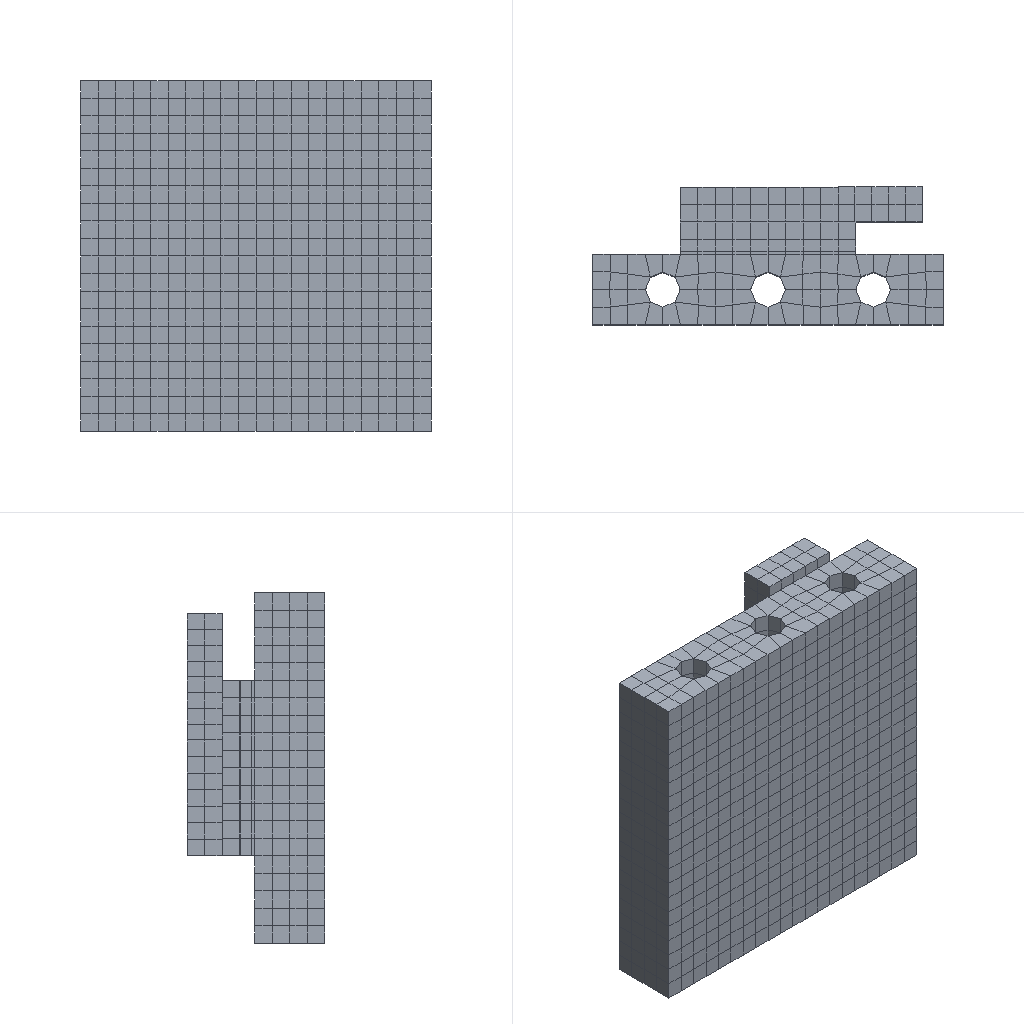Simulation study | ansys workbench
Set-up summary:
category,name,step,type,value,unit,region
solver,ansys_workbench
units,SI m-kg-s (Pa),,stated,"/units,MKS"
analysis,LS1,,steady-state thermal
load_step,LS1,LS1,steady-state thermal,nsubst=1; time=1
mesh,nodes,,,12761
mesh,elements,,,5722
element_type,SOLID279,,,2036
element_type,SURF152,,,1276
element_type,TARGE170,,,1205
element_type,CONTA174,,,1205
material,Cu,,E,1.15e+11,Pa
material,Cu,,nu,0.34
material,Cu,,density,8960,kg m^-3
material,Cu,,conductivity,397,W m^-1 C^-1
material,Cu,,specific_heat,385,J kg^-1 C^-1
material,Cu,,cte,1.75e-05,C^-1
material,?,,E,3.25e+11,Pa
material,?,,nu,0.29
material,?,,density,10220,kg m^-3
material,?,,conductivity,138,W m^-1 C^-1
material,?,,specific_heat,251,J kg^-1 C^-1
material,?,,cte,5.1e-06,C^-1
material,Ag,,E,8.3e+10,Pa
material,Ag,,nu,0.37
material,Ag,,density,10490,kg m^-3
material,Ag,,conductivity,429,W m^-1 C^-1
material,Ag,,specific_heat,237,J kg^-1 C^-1
material,Ag,,cte,1.89e-05,C^-1
material,SiC,,E,4.1e+11,Pa
material,SiC,,nu,0.25
material,SiC,,density,3200,kg m^-3
material,SiC,,conductivity,490,W m^-1 C^-1
material,SiC,,specific_heat,840,J kg^-1 C^-1
material,SiC,,cte,4.5e-06,C^-1
load,Define Uniform Initial temperature,model,body load temp,22,,all
load,"Create ""?""",LS1,heat flux,400000,,SURF152 #19
load,"Create ""______""",LS1,convection,15,,SURF152 #20
load,"Create ""______ 2""",LS1,convection,1000,,SURF152 #21
contact,Contact Region,,bonded (always),element=CONTA174
contact,Contact Region 2,,bonded (always),element=CONTA174
contact,Contact Region 3,,bonded (always),element=CONTA174
contact,Contact Region 4,,bonded (always),element=CONTA174
contact,Contact Region 5,,bonded (always),element=CONTA174
contact,Contact Region 6,,bonded (always),element=CONTA174
Ansys APDL input file, long lists of numbers shortened:
/batch
/config,noeldb,1     ! force off writing results to database
*get,_wallstrt,active,,time,wall
! ANSYS input file written by Workbench version 2021 R1
! File used for geometry attach:
/title,wbnew--___ (B5)
! ****** Begin Custom Load Command Snippet ******
/COM, ACT Extensions:
/COM,     LSDYNA, 2021.1
/COM,
! ****** End   Custom Load Command Snippet ******
*DIM,_wb_ProjectScratch_dir,string,248
_wb_ProjectScratch_dir(1) = ''
*DIM,_wb_SolverFiles_dir,string,248
_wb_SolverFiles_dir(1) = ''
*DIM,_wb_userfiles_dir,string,248
_wb_userfiles_dir(1) = ''
/com,--- Data in consistent MKS units. See Solving Units in the help system for more information.
/units,MKS
/nopr
/wb,file,start              !  signify a WB generated input file
/prep7
! Turn off shape checking because checks already performed inside WB mesher.
! See help system for more information.
SHPP,OFF,,NOWARN
/nolist
etcon,set             ! allow ANSYS to choose best KEYOP's for 180x elements, resets any applicable keyopt to MAPDL defaults
/com,*********** Nodes for the whole assembly ***********
nblock,3,,14037
(1i9,3e20.9e3)
        1    -4.290009604E-03    -4.526208412E-03     1.012469869E+00
! (12760 more lines like these left out)
-1
/wb,elem,start            !  set before creation of elements
/com,*********** Elements for Body 1 "DBC___|__(__)1" ***********
et,1,279
eblock,19,solid,,1360
(19i9)
        1        1        1        1        0        0        0        0       20        0      677     5025     5672     5732     5519     5564     5727     5728     5538
! (2719 more lines like these left out)
-1
/com,*********** Elements for Body 2 "mo|__-__1" ***********
et,2,279
eblock,19,solid,,100
(19i9)
        2        2        2        2        0        0        0        0       20        0      101      884     1025     1026     1027      885      986      985      984
! (199 more lines like these left out)
-1
/com,*********** Elements for Body 3 "___|__-__1" ***********
et,3,279
eblock,19,solid,,100
(19i9)
        3        3        3        3        0        0        0        0       20        0      301     2490     2631     2632     2633     2491     2592     2591     2590
! (199 more lines like these left out)
-1
/com,*********** Elements for Body 4 "__|__-__2" ***********
et,4,279
eblock,19,solid,,276
(19i9)
        4        4        4        4        0        0        0        0       20        0      401     3213     3691     3684     3675     3432     3692     3683     3682
! (551 more lines like these left out)
-1
/com,*********** Elements for Body 5 "__|__-__1" ***********
et,5,279
eblock,19,solid,,100
(19i9)
        5        5        5        5        0        0        0        0       20        0        1       81      214      223      232       82      190      191      172
! (199 more lines like these left out)
-1
/com,*********** Elements for Body 6 "__|__-__2" ***********
et,6,279
eblock,19,solid,,100
(19i9)
        6        6        6        6        0        0        0        0       20        0      201     1687     1828     1829     1830     1688     1789     1788     1787
! (199 more lines like these left out)
-1
/wb,elem,end               !  done creating elements
/com,*********** Send User Defined Coordinate System(s) ***********
csys,0
toffst,273.15,  ! Temperature offset from absolute zero
/wb,mat,start              !  starting to send materials
/com,*********** Send Materials ***********
MP,DENS,1,8960,	! kg m^-3
MP,ALPX,1,1.75e-05,	! C^-1
MP,EX,1,115000000000,	! Pa
MP,NUXY,1,0.34,
! (32 more lines like these left out)
/wb,mat,end                !  done sending materials
!************************* Model Summary ********************
!DBC___|__(__)1,	Cu,	matid,	1
!mo|__-__1,	钼,	matid,	2
!___|__-__1,	Ag,	matid,	3
!__|__-__2,	Cu,	matid,	4
!__|__-__1,	SiC,	matid,	5
!__|__-__2,	SiC,	matid,	6
!************************* End Model Summary ********************
! get the diagonal of the bounding box. Needed later for other things
*get,_xmin,node,,mnloc,x
*get,_ymin,node,,mnloc,y
*get,_zmin,node,,mnloc,z
*get,_xmax,node,,mxloc,x
*get,_ymax,node,,mxloc,y
*get,_zmax,node,,mxloc,z
_ASMDIAG=(_xmax-_xmin)*(_xmax-_xmin)+(_ymax-_ymin)*(_ymax-_ymin)+(_zmax-_zmin)*(_zmax-_zmin)
_ASMDIAG=SQRT(_ASMDIAG)
/wb,contact,start          !  starting to send contact
/com,*********** Create Contact "接触区域" ***********
/com,            Real Constant Set For Above Contact Is 8 & 7
*set,tid,8
*set,cid,7
r,tid
r,cid
et,tid,170
et,cid,174
eblock,10,,,144
(15i9)
     4965        8        8        8        0     6309     6310     6291     6290    11184    11144    11141    11142
! (143 more lines like these left out)
-1
eblock,10,,,144
(15i9)
     5109        7        7        7        0     6309     6310     6291     6290    11184    11144    11141    11142
! (143 more lines like these left out)
-1
eblock,10,,,100
(15i9)
     5253        7        8        7        0     2631     2490     2633     2632     2911     2912     3194     3193
! (99 more lines like these left out)
-1
eblock,10,,,100
(15i9)
     5353        8        7        8        0     2631     2490     2633     2632     2911     2912     3194     3193
! (99 more lines like these left out)
-1
keyo,cid,8,2               ! auto create asymmetric contact (from Program Controlled setting)
keyo,cid,10,0              ! adjust contact stiffness each NR iteration (from Program Controlled setting)
keyo,cid,12,5              ! bonded always
keyo,cid,18,1              ! small sliding turned on by application
keyo,cid,2,0               ! augmented Lagrange (from Program Controlled setting)
keyo,cid,4,0               ! on Gauss point (from Program Controlled setting)
keyo,cid,9,1               ! ignore initial gaps/penetration
keyo,cid,7,0               ! No Prediction
rmod,tid,3,10.      ! FKN
rmod,tid,5,0.       ! ICONT
rmod,tid,6,0.       ! PINB
rmod,tid,10,0.      ! CNOF
rmod,tid,12,0.      ! FKT
rmod,tid,36,42      ! WB DSID
rmod,cid,3,10.      ! FKN
rmod,cid,5,0.       ! ICONT
rmod,cid,6,0.       ! PINB
rmod,cid,10,0.      ! CNOF
rmod,cid,12,0.      ! FKT
rmod,cid,36,42      ! WB DSID
*set,_maxkxx,4900000.
rmod,cid,14,_maxkxx/_ASMDIAG         ! TCC, Divide by Length since Traction Based
rmod,tid,14,_maxkxx/_ASMDIAG      ! TCC, Divide by Length since Traction Based
keyo,cid,1,2     ! Pure thermal contact
/com,*********** Create Contact "接触区域 2" ***********
/com,            Real Constant Set For Above Contact Is 10 & 9
*set,tid,10
*set,cid,9
r,tid
r,cid
et,tid,170
et,cid,174
eblock,10,,,76
(15i9)
     5453       10       10       10        0      984      885      986      985     1309     1310     1526     1524
! (75 more lines like these left out)
-1
eblock,10,,,76
(15i9)
     5529        9        9        9        0      984      885      986      985     1309     1310     1526     1524
! (75 more lines like these left out)
-1
eblock,10,,,85
(15i9)
     5605        9       10        9        0     3554     3449     3445     3555     4473     4463     4464     4701
! (84 more lines like these left out)
-1
eblock,10,,,85
(15i9)
     5690       10        9       10        0     3554     3449     3445     3555     4473     4463     4464     4701
! (84 more lines like these left out)
-1
keyo,cid,8,2               ! auto create asymmetric contact (from Program Controlled setting)
keyo,cid,10,0              ! adjust contact stiffness each NR iteration (from Program Controlled setting)
keyo,cid,12,5              ! bonded always
keyo,cid,18,1              ! small sliding turned on by application
keyo,cid,2,0               ! augmented Lagrange (from Program Controlled setting)
keyo,cid,4,0               ! on Gauss point (from Program Controlled setting)
keyo,cid,9,1               ! ignore initial gaps/penetration
keyo,cid,7,0               ! No Prediction
rmod,tid,3,10.      ! FKN
rmod,tid,5,0.       ! ICONT
rmod,tid,6,0.       ! PINB
rmod,tid,10,0.      ! CNOF
rmod,tid,12,0.      ! FKT
rmod,tid,36,45      ! WB DSID
rmod,cid,3,10.      ! FKN
rmod,cid,5,0.       ! ICONT
rmod,cid,6,0.       ! PINB
rmod,cid,10,0.      ! CNOF
rmod,cid,12,0.      ! FKT
rmod,cid,36,45      ! WB DSID
*set,_maxkxx,4900000.
rmod,cid,14,_maxkxx/_ASMDIAG         ! TCC, Divide by Length since Traction Based
rmod,tid,14,_maxkxx/_ASMDIAG      ! TCC, Divide by Length since Traction Based
keyo,cid,1,2     ! Pure thermal contact
/com,*********** Create Contact "接触区域 3" ***********
/com,            Real Constant Set For Above Contact Is 12 & 11
*set,tid,12
*set,cid,11
r,tid
r,cid
et,tid,170
et,cid,174
eblock,10,,,100
(15i9)
     5775       12       12       12        0     1025      884     1027     1026     1305     1306     1588     1587
! (99 more lines like these left out)
-1
eblock,10,,,100
(15i9)
     5875       11       11       11        0     1025      884     1027     1026     1305     1306     1588     1587
! (99 more lines like these left out)
-1
eblock,10,,,100
(15i9)
     5975       11       12       11        0      172       82      190      191      506      507      740      704
! (99 more lines like these left out)
-1
eblock,10,,,100
(15i9)
     6075       12       11       12        0      172       82      190      191      506      507      740      704
! (99 more lines like these left out)
-1
keyo,cid,8,2               ! auto create asymmetric contact (from Program Controlled setting)
keyo,cid,10,0              ! adjust contact stiffness each NR iteration (from Program Controlled setting)
keyo,cid,12,5              ! bonded always
keyo,cid,18,1              ! small sliding turned on by application
keyo,cid,2,0               ! augmented Lagrange (from Program Controlled setting)
keyo,cid,4,0               ! on Gauss point (from Program Controlled setting)
keyo,cid,9,1               ! ignore initial gaps/penetration
keyo,cid,7,0               ! No Prediction
rmod,tid,3,10.      ! FKN
rmod,tid,5,0.       ! ICONT
rmod,tid,6,0.       ! PINB
rmod,tid,10,0.      ! CNOF
rmod,tid,12,0.      ! FKT
rmod,tid,36,48      ! WB DSID
rmod,cid,3,10.      ! FKN
rmod,cid,5,0.       ! ICONT
rmod,cid,6,0.       ! PINB
rmod,cid,10,0.      ! CNOF
rmod,cid,12,0.      ! FKT
rmod,cid,36,48      ! WB DSID
*set,_maxkxx,4900000.
rmod,cid,14,_maxkxx/_ASMDIAG         ! TCC, Divide by Length since Traction Based
rmod,tid,14,_maxkxx/_ASMDIAG      ! TCC, Divide by Length since Traction Based
keyo,cid,1,2     ! Pure thermal contact
/com,*********** Create Contact "接触区域 4" ***********
/com,            Real Constant Set For Above Contact Is 14 & 13
*set,tid,14
*set,cid,13
r,tid
r,cid
et,tid,170
et,cid,174
eblock,10,,,100
(15i9)
     6175       14       14       14        0     1025      884     1027     1026     1305     1306     1588     1587
! (99 more lines like these left out)
-1
eblock,10,,,100
(15i9)
     6275       13       13       13        0     1025      884     1027     1026     1305     1306     1588     1587
! (99 more lines like these left out)
-1
eblock,10,,,100
(15i9)
     6375       13       14       13        0     1787     1688     1789     1788     2112     2113     2329     2327
! (99 more lines like these left out)
-1
eblock,10,,,100
(15i9)
     6475       14       13       14        0     1787     1688     1789     1788     2112     2113     2329     2327
! (99 more lines like these left out)
-1
keyo,cid,8,2               ! auto create asymmetric contact (from Program Controlled setting)
keyo,cid,10,0              ! adjust contact stiffness each NR iteration (from Program Controlled setting)
keyo,cid,12,5              ! bonded always
keyo,cid,18,1              ! small sliding turned on by application
keyo,cid,2,0               ! augmented Lagrange (from Program Controlled setting)
keyo,cid,4,0               ! on Gauss point (from Program Controlled setting)
keyo,cid,9,1               ! ignore initial gaps/penetration
keyo,cid,7,0               ! No Prediction
rmod,tid,3,10.      ! FKN
rmod,tid,5,0.       ! ICONT
rmod,tid,6,0.       ! PINB
rmod,tid,10,0.      ! CNOF
rmod,tid,12,0.      ! FKT
rmod,tid,36,51      ! WB DSID
rmod,cid,3,10.      ! FKN
rmod,cid,5,0.       ! ICONT
rmod,cid,6,0.       ! PINB
rmod,cid,10,0.      ! CNOF
rmod,cid,12,0.      ! FKT
rmod,cid,36,51      ! WB DSID
*set,_maxkxx,4900000.
rmod,cid,14,_maxkxx/_ASMDIAG         ! TCC, Divide by Length since Traction Based
rmod,tid,14,_maxkxx/_ASMDIAG      ! TCC, Divide by Length since Traction Based
keyo,cid,1,2     ! Pure thermal contact
/com,*********** Create Contact "接触区域 5" ***********
/com,            Real Constant Set For Above Contact Is 16 & 15
*set,tid,16
*set,cid,15
r,tid
r,cid
et,tid,170
et,cid,174
eblock,10,,,100
(15i9)
     6575       16       16       16        0     2590     2491     2592     2591     2915     2916     3132     3130
! (99 more lines like these left out)
-1
eblock,10,,,100
(15i9)
     6675       15       15       15        0     2590     2491     2592     2591     2915     2916     3132     3130
! (99 more lines like these left out)
-1
eblock,10,,,100
(15i9)
     6775       15       16       15        0      214       81      232      223      502      503      785      777
! (99 more lines like these left out)
-1
eblock,10,,,100
(15i9)
     6875       16       15       16        0      214       81      232      223      502      503      785      777
! (99 more lines like these left out)
-1
keyo,cid,8,2               ! auto create asymmetric contact (from Program Controlled setting)
keyo,cid,10,0              ! adjust contact stiffness each NR iteration (from Program Controlled setting)
keyo,cid,12,5              ! bonded always
keyo,cid,18,1              ! small sliding turned on by application
keyo,cid,2,0               ! augmented Lagrange (from Program Controlled setting)
keyo,cid,4,0               ! on Gauss point (from Program Controlled setting)
keyo,cid,9,1               ! ignore initial gaps/penetration
keyo,cid,7,0               ! No Prediction
rmod,tid,3,10.      ! FKN
rmod,tid,5,0.       ! ICONT
rmod,tid,6,0.       ! PINB
rmod,tid,10,0.      ! CNOF
rmod,tid,12,0.      ! FKT
rmod,tid,36,54      ! WB DSID
rmod,cid,3,10.      ! FKN
rmod,cid,5,0.       ! ICONT
rmod,cid,6,0.       ! PINB
rmod,cid,10,0.      ! CNOF
rmod,cid,12,0.      ! FKT
rmod,cid,36,54      ! WB DSID
*set,_maxkxx,4900000.
rmod,cid,14,_maxkxx/_ASMDIAG         ! TCC, Divide by Length since Traction Based
rmod,tid,14,_maxkxx/_ASMDIAG      ! TCC, Divide by Length since Traction Based
keyo,cid,1,2     ! Pure thermal contact
/com,*********** Create Contact "接触区域 6" ***********
/com,            Real Constant Set For Above Contact Is 18 & 17
*set,tid,18
*set,cid,17
r,tid
r,cid
et,tid,170
et,cid,174
eblock,10,,,100
(15i9)
     6975       18       18       18        0      172       82      190      191      506      507      740      704
! (99 more lines like these left out)
-1
eblock,10,,,100
(15i9)
     7075       17       17       17        0      172       82      190      191      506      507      740      704
! (99 more lines like these left out)
-1
eblock,10,,,100
(15i9)
     7175       17       18       17        0     1828     1687     1830     1829     2108     2109     2391     2390
! (99 more lines like these left out)
-1
eblock,10,,,100
(15i9)
     7275       18       17       18        0     1828     1687     1830     1829     2108     2109     2391     2390
! (99 more lines like these left out)
-1
keyo,cid,8,2               ! auto create asymmetric contact (from Program Controlled setting)
keyo,cid,10,0              ! adjust contact stiffness each NR iteration (from Program Controlled setting)
keyo,cid,12,5              ! bonded always
keyo,cid,18,1              ! small sliding turned on by application
keyo,cid,2,0               ! augmented Lagrange (from Program Controlled setting)
keyo,cid,4,0               ! on Gauss point (from Program Controlled setting)
keyo,cid,9,1               ! ignore initial gaps/penetration
keyo,cid,7,0               ! No Prediction
rmod,tid,3,10.      ! FKN
rmod,tid,5,0.       ! ICONT
rmod,tid,6,0.       ! PINB
rmod,tid,10,0.      ! CNOF
rmod,tid,12,0.      ! FKT
rmod,tid,36,57      ! WB DSID
rmod,cid,3,10.      ! FKN
rmod,cid,5,0.       ! ICONT
rmod,cid,6,0.       ! PINB
rmod,cid,10,0.      ! CNOF
rmod,cid,12,0.      ! FKT
rmod,cid,36,57      ! WB DSID
*set,_maxkxx,4900000.
rmod,cid,14,_maxkxx/_ASMDIAG         ! TCC, Divide by Length since Traction Based
rmod,tid,14,_maxkxx/_ASMDIAG      ! TCC, Divide by Length since Traction Based
keyo,cid,1,2     ! Pure thermal contact
nsel,all
esel,all
/wb,contact,end            !  done creating contacts
/golist
/wb,load,start             !  starting to send loads
/com,*********** Create "热流" ***********
et,19,152
eblock,10,,,100
(15i9)
     7375       19       19       19        0      172       82      190      191      506      507      740      704
! (99 more lines like these left out)
-1
esel,s,type,,19
keyop,19,8,1      ! include heat flux
esel,all
fcum,add                   ! add nodal forces up (needed in case have loads on the same edge,vertex)
nsel,all
nsel,all
fcum                       ! reset default on fcum command since done sending WB F loads
/com,*********** Create "______" ***********
et,20,152
eblock,10,,,696
(15i9)
     7475       20       20       20        0     5669     5571     5597     5668     9363     9361     9431     9591
! (695 more lines like these left out)
-1
esel,s,type,,20
keyop,20,8,2.
keyop,20,13,0
/com,*********** Create "______ 2" ***********
et,21,152
eblock,10,,,480
(15i9)
     8171       21       21       21        0     5951     5870     5930     5931    10147    10146    10341    10343
! (479 more lines like these left out)
-1
esel,s,type,,21
keyop,21,8,2.
keyop,21,13,0
esel,all
/com,***************** Define Uniform Initial temperature ***************
tunif,22.
/gst,on,on
fini
*get,_numnode,node,0,count
*get,_numelem,elem,0,count
*get, _MAXELEMNUM, elem, 0, NUM, MAX
*get, _MAXNODENUM, node, 0, NUM, MAX
*get, _MAXELEMTYPE, etyp, 0, NUM, MAX
*get, _MAXREALCONST, real, 0, NUM, MAX
/go
/wb,load,end               !  done creating loads
/com,--- Number of total nodes = %_numnode%
/com,--- Number of contact elements = 3686
/com,--- Number of spring elements = 0
/com,--- Number of bearing elements = 0
/com,--- Number of solid elements = 2036
/com,--- Number of condensed parts = 0
/com,--- Number of total elements = %_numelem%
*get,_wallbsol,active,,time,wall
/com,****************************************************************************
/com,*************************    SOLUTION       ********************************
/com,****************************************************************************
/solu
antype,0                   ! static analysis
!eqsl,sparse               ! using sparse solver which is default so no eqsl command needed
cntr,print,1               ! print out contact info and also make no initial contact an error
rescontrol,,none                 ! Do not keep any restart files
dmpoption,emat,no             ! Don't combine emat file for DANSYS
dmpoption,esav,no             ! Don't combine esav file for DANSYS
/com,****************************************************
/com,******************* SOLVE FOR LS 1 OF 1 ****************
esel,s,type,,19
nsle
sf,all,hflux,400000.
nsel,all
esel,all
esel,s,type,,20
nsle
sf,all,conv,15.,22.
esel,s,type,,21
nsle
sf,all,conv,1000.,22.
nsel,all
esel,all
autots,on
nsub,1,10,1
time,1.
outres,erase
outres,all,none
outres,nsol,all
outres,rsol,all
outres,eangl,all
outres,veng,all
outres,fflux,all
outres,cont,all
/nopr
esel,s,type,,20
esel,a,type,,21
cm,_elmisc,elem
esel,all
/gopr
outres,misc,all,_elmisc
cnvtol,heat,,.001,,1.e-006    ! Program Controlled. Set MINREF equivalent of 1e-6 Watts
! *********** WB SOLVE COMMAND ***********
! check interactive state
*get,ANSINTER_,active,,int
*if,ANSINTER_,ne,0,then
/eof
*endif
solve
/com *************** Write FE CONNECTORS *********
CEWRITE,file,ce,,INTE
/com,****************************************************
/com,*************** FINISHED SOLVE FOR LS 1 *************
*get,_wallasol,active,,time,wall
/post1
xmlo,ENCODING,ISO-8859-1
xmlo,parm
/xml,parm,xml
fini
/gopr
*get,_walldone,active,,time,wall
_preptime=(_wallbsol-_wallstrt)*3600
_solvtime=(_wallasol-_wallbsol)*3600
_posttime=(_walldone-_wallasol)*3600
_totaltim=(_walldone-_wallstrt)*3600
*get,_dlbratio,active,0,solu,dlbr
*get,_combtime,active,0,solu,comb
/com,--- Total number of nodes = %_numnode%
/com,--- Total number of elements = %_numelem%
/com,--- Element load balance ratio = %_dlbratio%
/com,--- Time to combine distributed files = %_combtime%
/wb,file,end               ! done with WB generated input
Results summary:
result,analyses[0].index,,,1
result,analyses[0].system,,,SYS-2
result,analyses[0].deck,,,deck.dat
result,analyses[0].solve_status,,,completed
result,analyses[0].analysis_type,,,static
result,analyses[0].physics,,,thermal
result,analyses[0].unit_system,,,"MKS: m, kg, N, s, V, A, degC"
result,analyses[0].n_sets,,,1
result,analyses[0].load_steps[0].set,set=1,,1
result,analyses[0].load_steps[0].time_or_freq,set=1,,1
result,analyses[0].load_steps[0].max_temperature,set=1,,127.189
result,analyses[0].load_steps[0].min_temperature,set=1,,124.671
result,geometry_export[0][0],,,.step
result,geometry_export[0][1],,,ok
result,geometry_export[0][2],,,6